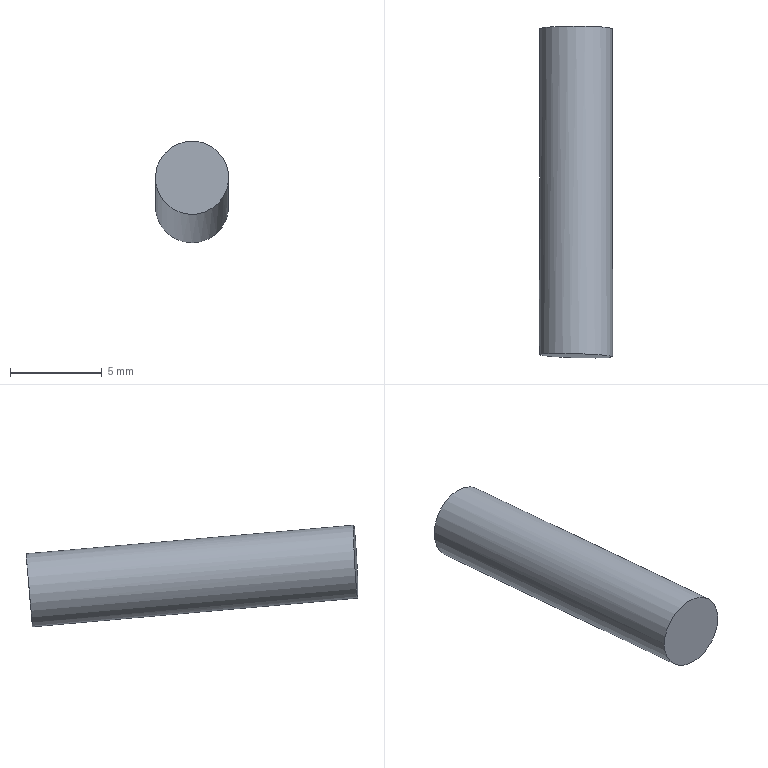Part | NX | features solid 2 | 1 solid | 3 faces | box 4 x 18.111 x 5.549 mm | volume 224.713 mm3 | plane 2 | cylinder 1 | commonest cylinder face diameters 4 x1
STEP:
#1=CARTESIAN_POINT('',(280.775,-41.544,-42.274));
#2=VERTEX_POINT('',#1);
#3=CARTESIAN_POINT('',(280.775,-41.37,-40.281));
#4=DIRECTION('',(0.,-0.9962,0.08716));
#5=DIRECTION('',(0.,-0.08716,-0.9962));
#6=AXIS2_PLACEMENT_3D('',#3,#4,#5);
#7=CIRCLE('',#6,2.);
#8=EDGE_CURVE('',#2,#2,#7,.T.);
#9=ORIENTED_EDGE('',*,*,#8,.F.);
#10=EDGE_LOOP('',(#9));
#11=FACE_BOUND('',#10,.T.);
#12=CARTESIAN_POINT('',(280.775,-41.37,-40.281));
#13=DIRECTION('',(0.,0.9962,-0.08716));
#14=DIRECTION('',(0.,0.08716,0.9962));
#15=AXIS2_PLACEMENT_3D('',#12,#13,#14);
#16=PLANE('',#15);
#17=ADVANCED_FACE('',(#11),#16,.T.);
#18=CARTESIAN_POINT('',(279.435,-59.222,-40.21));
#19=VERTEX_POINT('',#18);
#20=CARTESIAN_POINT('',(280.775,-59.184,-38.723));
#21=DIRECTION('',(0.03046,0.9981,-0.05344));
#22=DIRECTION('',(-0.6692,-0.01935,-0.7428));
#23=AXIS2_PLACEMENT_3D('',#20,#21,#22);
#24=ELLIPSE('',#23,2.002,2.);
#25=EDGE_CURVE('',#19,#19,#24,.T.);
#26=ORIENTED_EDGE('',*,*,#25,.F.);
#27=EDGE_LOOP('',(#26));
#28=FACE_BOUND('',#27,.T.);
#29=CARTESIAN_POINT('',(457.994,-68.531,-112.302));
#30=DIRECTION('',(0.03046,0.9981,-0.05344));
#31=DIRECTION('',(0.06614,0.05134,0.9965));
#32=AXIS2_PLACEMENT_3D('',#29,#30,#31);
#33=PLANE('',#32);
#34=ADVANCED_FACE('',(#28),#33,.F.);
#35=ORIENTED_EDGE('',*,*,#8,.T.);
#36=EDGE_LOOP('',(#35));
#37=FACE_BOUND('',#36,.T.);
#38=ORIENTED_EDGE('',*,*,#25,.T.);
#39=EDGE_LOOP('',(#38));
#40=FACE_BOUND('',#39,.T.);
#41=CARTESIAN_POINT('',(280.775,-61.294,-38.538));
#42=DIRECTION('',(0.,0.9962,-0.08716));
#43=DIRECTION('',(0.,0.08716,0.9962));
#44=AXIS2_PLACEMENT_3D('',#41,#42,#43);
#45=CYLINDRICAL_SURFACE('',#44,2.);
#46=ADVANCED_FACE('',(#37,#40),#45,.T.);
#47=CLOSED_SHELL('',(#17,#34,#46));
#48=MANIFOLD_SOLID_BREP('',#47);
#49=(LENGTH_UNIT()NAMED_UNIT(*)SI_UNIT(.MILLI.,.METRE.));
#50=UNCERTAINTY_MEASURE_WITH_UNIT(LENGTH_MEASURE(0.00001),#49,'','');
#51=(NAMED_UNIT(*)PLANE_ANGLE_UNIT()SI_UNIT($,.RADIAN.));
#52=(NAMED_UNIT(*)SI_UNIT($,.STERADIAN.)SOLID_ANGLE_UNIT());
#53=(GEOMETRIC_REPRESENTATION_CONTEXT(3)GLOBAL_UNCERTAINTY_ASSIGNED_CONTEXT((#50))GLOBAL_UNIT_ASSIGNED_CONTEXT((#49,#51,#52))REPRESENTATION_CONTEXT('',''));
#54=ADVANCED_BREP_SHAPE_REPRESENTATION('',(#48),#53);